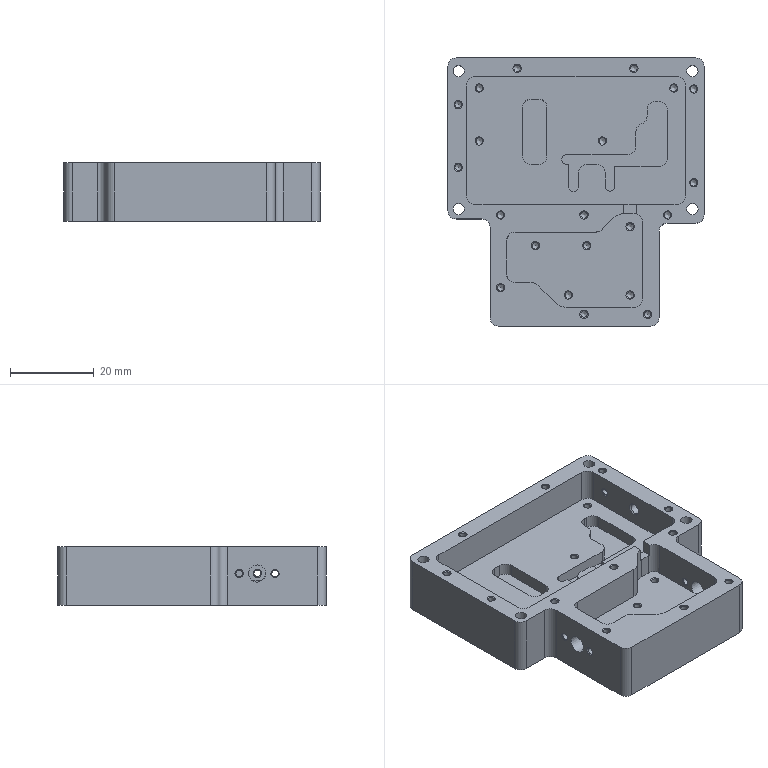Part | STEP file | Front stage cavity | 1 solid | 167 faces | box 61.4 x 64.23 x 14 mm | volume 29019 mm3 | cylinder 68 | cone 52 | plane 47 | commonest cylinder face diameters 4 x28 1.6 x26 2.7 x4 2.311 x3 4.1 x2 5.132 x2